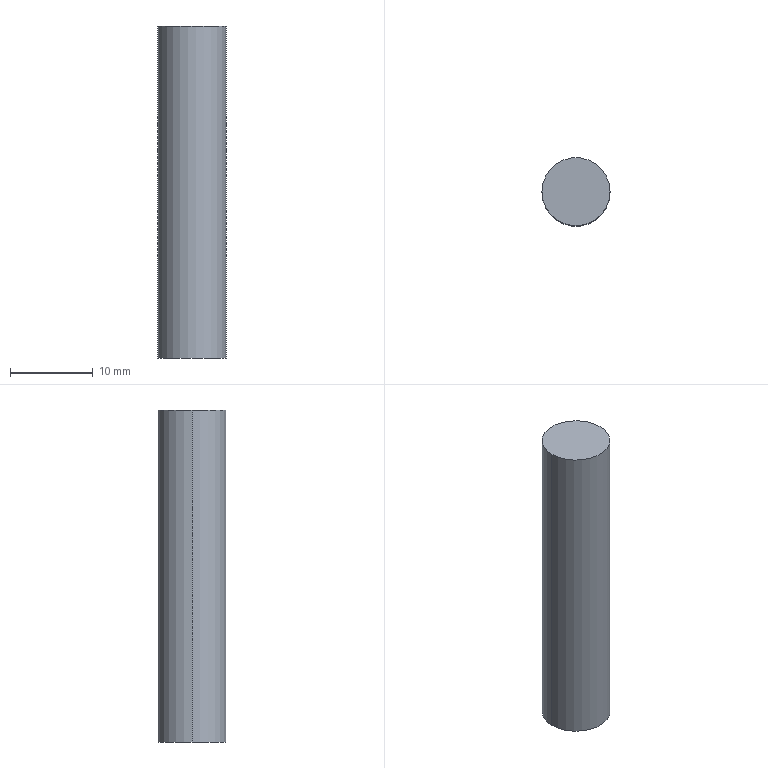Part | STEP file | X-axis cable carrier wiring-Part-32 | 1 solid | 4 faces | box 8.2 x 8.2 x 40 mm | volume 2112 mm3 | cylinder 2 | plane 2 | commonest cylinder face diameters 8.2 x2
STEP:
#1=CARTESIAN_POINT('',(0.,0.,0.));
#2=DIRECTION('',(0.,0.,1.));
#3=DIRECTION('',(1.,0.,0.));
#4=AXIS2_PLACEMENT_3D('',#1,#2,#3);
#5=CARTESIAN_POINT('',(185.,4.1,0.));
#6=VERTEX_POINT('',#5);
#7=CARTESIAN_POINT('',(176.8,4.1,0.));
#8=VERTEX_POINT('',#7);
#9=CARTESIAN_POINT('',(180.9,4.1,0.));
#10=DIRECTION('',(0.,0.,1.));
#11=DIRECTION('',(1.,0.,0.));
#12=AXIS2_PLACEMENT_3D('',#9,#10,#11);
#13=CIRCLE('',#12,4.1);
#14=CARTESIAN_POINT('',(180.9,4.1,0.));
#15=DIRECTION('',(0.,0.,1.));
#16=DIRECTION('',(1.,0.,0.));
#17=AXIS2_PLACEMENT_3D('',#14,#15,#16);
#18=CYLINDRICAL_SURFACE('',#17,4.1);
#19=CARTESIAN_POINT('',(0.,0.));
#20=DIRECTION('',(1.,0.));
#21=VECTOR('',#20,1.);
#22=LINE('',#19,#21);
#23=(GEOMETRIC_REPRESENTATION_CONTEXT(2)PARAMETRIC_REPRESENTATION_CONTEXT()REPRESENTATION_CONTEXT('',''));
#24=DEFINITIONAL_REPRESENTATION('',(#22),#23);
#25=PCURVE('',#18,#24);
#26=CARTESIAN_POINT('',(180.9,4.1,0.));
#27=DIRECTION('',(0.,0.,-1.));
#28=DIRECTION('',(-1.,0.,0.));
#29=AXIS2_PLACEMENT_3D('',#26,#27,#28);
#30=PLANE('',#29);
#31=CARTESIAN_POINT('',(-4.1,0.));
#32=CARTESIAN_POINT('',(-4.1,7.101));
#33=CARTESIAN_POINT('',(2.05,3.551));
#34=CARTESIAN_POINT('',(8.2,0.));
#35=CARTESIAN_POINT('',(2.05,-3.551));
#36=CARTESIAN_POINT('',(-4.1,-7.101));
#37=CARTESIAN_POINT('',(-4.1,0.));
#38=(BOUNDED_CURVE()B_SPLINE_CURVE(2,(#31,#32,#33,#34,#35,#36,#37),.UNSPECIFIED.,.T.,.F.)B_SPLINE_CURVE_WITH_KNOTS((1,2,2,2,2,1),(-2.094,0.,2.094,4.189,6.283,8.378),.UNSPECIFIED.)CURVE()GEOMETRIC_REPRESENTATION_ITEM()RATIONAL_B_SPLINE_CURVE((1.,0.5,1.,0.5,1.,0.5,1.))REPRESENTATION_ITEM(''));
#39=(GEOMETRIC_REPRESENTATION_CONTEXT(2)PARAMETRIC_REPRESENTATION_CONTEXT()REPRESENTATION_CONTEXT('',''));
#40=DEFINITIONAL_REPRESENTATION('',(#38),#39);
#41=PCURVE('',#30,#40);
#42=SURFACE_CURVE('',#13,(#25,#41),.PCURVE_S1.);
#43=EDGE_CURVE('',#6,#8,#42,.T.);
#44=ORIENTED_EDGE('',*,*,#43,.T.);
#45=CARTESIAN_POINT('',(176.8,4.1,40.));
#46=VERTEX_POINT('',#45);
#47=CARTESIAN_POINT('',(176.8,4.1,0.));
#48=DIRECTION('',(0.,0.,1.));
#49=VECTOR('',#48,1.);
#50=LINE('',#47,#49);
#51=CARTESIAN_POINT('',(3.142,0.));
#52=DIRECTION('',(0.,1.));
#53=VECTOR('',#52,1.);
#54=LINE('',#51,#53);
#55=(GEOMETRIC_REPRESENTATION_CONTEXT(2)PARAMETRIC_REPRESENTATION_CONTEXT()REPRESENTATION_CONTEXT('',''));
#56=DEFINITIONAL_REPRESENTATION('',(#54),#55);
#57=PCURVE('',#18,#56);
#58=CARTESIAN_POINT('',(180.9,4.1,0.));
#59=DIRECTION('',(0.,0.,1.));
#60=DIRECTION('',(1.,0.,0.));
#61=AXIS2_PLACEMENT_3D('',#58,#59,#60);
#62=CYLINDRICAL_SURFACE('',#61,4.1);
#63=CARTESIAN_POINT('',(3.142,0.));
#64=DIRECTION('',(0.,1.));
#65=VECTOR('',#64,1.);
#66=LINE('',#63,#65);
#67=(GEOMETRIC_REPRESENTATION_CONTEXT(2)PARAMETRIC_REPRESENTATION_CONTEXT()REPRESENTATION_CONTEXT('',''));
#68=DEFINITIONAL_REPRESENTATION('',(#66),#67);
#69=PCURVE('',#62,#68);
#70=SURFACE_CURVE('',#50,(#57,#69),.PCURVE_S1.);
#71=EDGE_CURVE('',#8,#46,#70,.T.);
#72=ORIENTED_EDGE('',*,*,#71,.T.);
#73=CARTESIAN_POINT('',(185.,4.1,40.));
#74=VERTEX_POINT('',#73);
#75=CARTESIAN_POINT('',(180.9,4.1,40.));
#76=DIRECTION('',(0.,0.,-1.));
#77=DIRECTION('',(-1.,0.,0.));
#78=AXIS2_PLACEMENT_3D('',#75,#76,#77);
#79=CIRCLE('',#78,4.1);
#80=CARTESIAN_POINT('',(3.142,40.));
#81=DIRECTION('',(-1.,0.));
#82=VECTOR('',#81,1.);
#83=LINE('',#80,#82);
#84=(GEOMETRIC_REPRESENTATION_CONTEXT(2)PARAMETRIC_REPRESENTATION_CONTEXT()REPRESENTATION_CONTEXT('',''));
#85=DEFINITIONAL_REPRESENTATION('',(#83),#84);
#86=PCURVE('',#18,#85);
#87=CARTESIAN_POINT('',(180.9,4.1,40.));
#88=DIRECTION('',(0.,0.,1.));
#89=DIRECTION('',(1.,0.,0.));
#90=AXIS2_PLACEMENT_3D('',#87,#88,#89);
#91=PLANE('',#90);
#92=CARTESIAN_POINT('',(-4.1,0.));
#93=CARTESIAN_POINT('',(-4.1,7.101));
#94=CARTESIAN_POINT('',(2.05,3.551));
#95=CARTESIAN_POINT('',(8.2,0.));
#96=CARTESIAN_POINT('',(2.05,-3.551));
#97=CARTESIAN_POINT('',(-4.1,-7.101));
#98=CARTESIAN_POINT('',(-4.1,0.));
#99=(BOUNDED_CURVE()B_SPLINE_CURVE(2,(#92,#93,#94,#95,#96,#97,#98),.UNSPECIFIED.,.T.,.F.)B_SPLINE_CURVE_WITH_KNOTS((1,2,2,2,2,1),(-2.094,0.,2.094,4.189,6.283,8.378),.UNSPECIFIED.)CURVE()GEOMETRIC_REPRESENTATION_ITEM()RATIONAL_B_SPLINE_CURVE((1.,0.5,1.,0.5,1.,0.5,1.))REPRESENTATION_ITEM(''));
#100=(GEOMETRIC_REPRESENTATION_CONTEXT(2)PARAMETRIC_REPRESENTATION_CONTEXT()REPRESENTATION_CONTEXT('',''));
#101=DEFINITIONAL_REPRESENTATION('',(#99),#100);
#102=PCURVE('',#91,#101);
#103=SURFACE_CURVE('',#79,(#86,#102),.PCURVE_S1.);
#104=EDGE_CURVE('',#46,#74,#103,.T.);
#105=ORIENTED_EDGE('',*,*,#104,.T.);
#106=CARTESIAN_POINT('',(185.,4.1,0.));
#107=DIRECTION('',(0.,0.,1.));
#108=VECTOR('',#107,1.);
#109=LINE('',#106,#108);
#110=CARTESIAN_POINT('',(0.,0.));
#111=DIRECTION('',(0.,1.));
#112=VECTOR('',#111,1.);
#113=LINE('',#110,#112);
#114=(GEOMETRIC_REPRESENTATION_CONTEXT(2)PARAMETRIC_REPRESENTATION_CONTEXT()REPRESENTATION_CONTEXT('',''));
#115=DEFINITIONAL_REPRESENTATION('',(#113),#114);
#116=PCURVE('',#18,#115);
#117=CARTESIAN_POINT('',(6.283,0.));
#118=DIRECTION('',(0.,1.));
#119=VECTOR('',#118,1.);
#120=LINE('',#117,#119);
#121=(GEOMETRIC_REPRESENTATION_CONTEXT(2)PARAMETRIC_REPRESENTATION_CONTEXT()REPRESENTATION_CONTEXT('',''));
#122=DEFINITIONAL_REPRESENTATION('',(#120),#121);
#123=PCURVE('',#62,#122);
#124=SURFACE_CURVE('',#109,(#116,#123),.PCURVE_S1.);
#125=EDGE_CURVE('',#6,#74,#124,.T.);
#126=ORIENTED_EDGE('',*,*,#125,.F.);
#127=EDGE_LOOP('',(#44,#72,#105,#126));
#128=FACE_BOUND('',#127,.T.);
#129=ADVANCED_FACE('',(#128),#18,.T.);
#130=CARTESIAN_POINT('',(180.9,4.1,40.));
#131=DIRECTION('',(0.,0.,-1.));
#132=DIRECTION('',(-1.,0.,0.));
#133=AXIS2_PLACEMENT_3D('',#130,#131,#132);
#134=CIRCLE('',#133,4.1);
#135=CARTESIAN_POINT('',(-4.1,0.));
#136=CARTESIAN_POINT('',(-4.1,7.101));
#137=CARTESIAN_POINT('',(2.05,3.551));
#138=CARTESIAN_POINT('',(8.2,0.));
#139=CARTESIAN_POINT('',(2.05,-3.551));
#140=CARTESIAN_POINT('',(-4.1,-7.101));
#141=CARTESIAN_POINT('',(-4.1,0.));
#142=(BOUNDED_CURVE()B_SPLINE_CURVE(2,(#135,#136,#137,#138,#139,#140,#141),.UNSPECIFIED.,.T.,.F.)B_SPLINE_CURVE_WITH_KNOTS((1,2,2,2,2,1),(-2.094,0.,2.094,4.189,6.283,8.378),.UNSPECIFIED.)CURVE()GEOMETRIC_REPRESENTATION_ITEM()RATIONAL_B_SPLINE_CURVE((1.,0.5,1.,0.5,1.,0.5,1.))REPRESENTATION_ITEM(''));
#143=(GEOMETRIC_REPRESENTATION_CONTEXT(2)PARAMETRIC_REPRESENTATION_CONTEXT()REPRESENTATION_CONTEXT('',''));
#144=DEFINITIONAL_REPRESENTATION('',(#142),#143);
#145=PCURVE('',#91,#144);
#146=CARTESIAN_POINT('',(9.425,40.));
#147=DIRECTION('',(-1.,0.));
#148=VECTOR('',#147,1.);
#149=LINE('',#146,#148);
#150=(GEOMETRIC_REPRESENTATION_CONTEXT(2)PARAMETRIC_REPRESENTATION_CONTEXT()REPRESENTATION_CONTEXT('',''));
#151=DEFINITIONAL_REPRESENTATION('',(#149),#150);
#152=PCURVE('',#62,#151);
#153=SURFACE_CURVE('',#134,(#145,#152),.PCURVE_S1.);
#154=EDGE_CURVE('',#74,#46,#153,.T.);
#155=ORIENTED_EDGE('',*,*,#154,.F.);
#156=ORIENTED_EDGE('',*,*,#104,.F.);
#157=EDGE_LOOP('',(#155,#156));
#158=FACE_BOUND('',#157,.T.);
#159=ADVANCED_FACE('',(#158),#91,.T.);
#160=ORIENTED_EDGE('',*,*,#43,.F.);
#161=CARTESIAN_POINT('',(180.9,4.1,0.));
#162=DIRECTION('',(0.,0.,1.));
#163=DIRECTION('',(1.,0.,0.));
#164=AXIS2_PLACEMENT_3D('',#161,#162,#163);
#165=CIRCLE('',#164,4.1);
#166=CARTESIAN_POINT('',(-4.1,0.));
#167=CARTESIAN_POINT('',(-4.1,7.101));
#168=CARTESIAN_POINT('',(2.05,3.551));
#169=CARTESIAN_POINT('',(8.2,0.));
#170=CARTESIAN_POINT('',(2.05,-3.551));
#171=CARTESIAN_POINT('',(-4.1,-7.101));
#172=CARTESIAN_POINT('',(-4.1,0.));
#173=(BOUNDED_CURVE()B_SPLINE_CURVE(2,(#166,#167,#168,#169,#170,#171,#172),.UNSPECIFIED.,.T.,.F.)B_SPLINE_CURVE_WITH_KNOTS((1,2,2,2,2,1),(-2.094,0.,2.094,4.189,6.283,8.378),.UNSPECIFIED.)CURVE()GEOMETRIC_REPRESENTATION_ITEM()RATIONAL_B_SPLINE_CURVE((1.,0.5,1.,0.5,1.,0.5,1.))REPRESENTATION_ITEM(''));
#174=(GEOMETRIC_REPRESENTATION_CONTEXT(2)PARAMETRIC_REPRESENTATION_CONTEXT()REPRESENTATION_CONTEXT('',''));
#175=DEFINITIONAL_REPRESENTATION('',(#173),#174);
#176=PCURVE('',#30,#175);
#177=CARTESIAN_POINT('',(0.,0.));
#178=DIRECTION('',(1.,0.));
#179=VECTOR('',#178,1.);
#180=LINE('',#177,#179);
#181=(GEOMETRIC_REPRESENTATION_CONTEXT(2)PARAMETRIC_REPRESENTATION_CONTEXT()REPRESENTATION_CONTEXT('',''));
#182=DEFINITIONAL_REPRESENTATION('',(#180),#181);
#183=PCURVE('',#62,#182);
#184=SURFACE_CURVE('',#165,(#176,#183),.PCURVE_S1.);
#185=EDGE_CURVE('',#8,#6,#184,.T.);
#186=ORIENTED_EDGE('',*,*,#185,.F.);
#187=EDGE_LOOP('',(#160,#186));
#188=FACE_BOUND('',#187,.T.);
#189=ADVANCED_FACE('',(#188),#30,.T.);
#190=ORIENTED_EDGE('',*,*,#71,.F.);
#191=ORIENTED_EDGE('',*,*,#185,.T.);
#192=ORIENTED_EDGE('',*,*,#125,.T.);
#193=ORIENTED_EDGE('',*,*,#154,.T.);
#194=EDGE_LOOP('',(#190,#191,#192,#193));
#195=FACE_BOUND('',#194,.T.);
#196=ADVANCED_FACE('',(#195),#62,.T.);
#197=CLOSED_SHELL('',(#129,#159,#189,#196));
#198=MANIFOLD_SOLID_BREP('',#197);
#199=(LENGTH_UNIT()NAMED_UNIT(*)SI_UNIT(.MILLI.,.METRE.));
#200=UNCERTAINTY_MEASURE_WITH_UNIT(LENGTH_MEASURE(0.0000001),#199,'','');
#201=(NAMED_UNIT(*)PLANE_ANGLE_UNIT()SI_UNIT($,.RADIAN.));
#202=(NAMED_UNIT(*)SI_UNIT($,.STERADIAN.)SOLID_ANGLE_UNIT());
#203=(GEOMETRIC_REPRESENTATION_CONTEXT(3)GLOBAL_UNCERTAINTY_ASSIGNED_CONTEXT((#200))GLOBAL_UNIT_ASSIGNED_CONTEXT((#199,#201,#202))REPRESENTATION_CONTEXT('',''));
#204=ADVANCED_BREP_SHAPE_REPRESENTATION('',(#4,#198),#203);